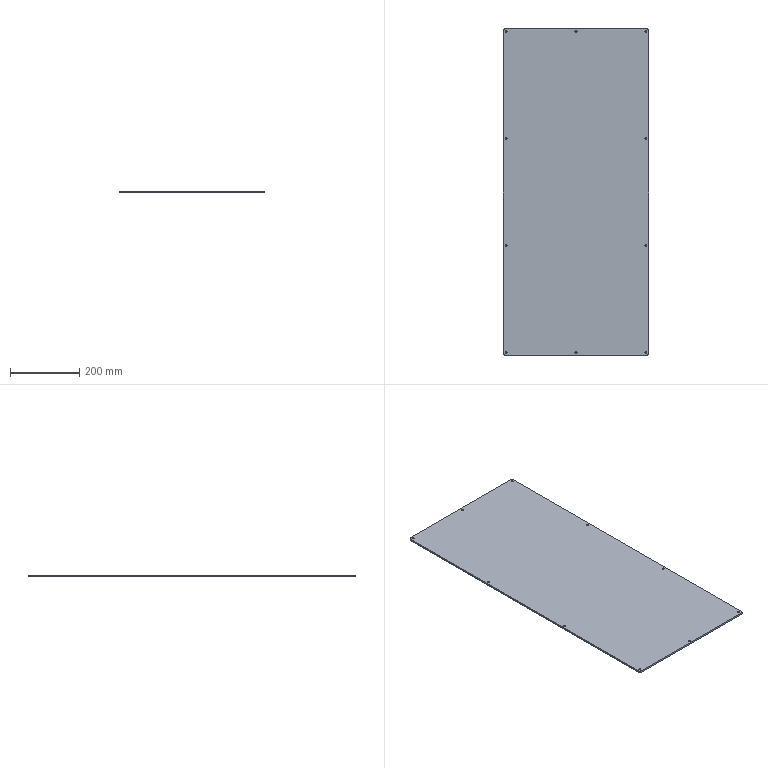Part | NX | features BREP 1 | 1 solid | 30 faces | box 421 x 944 x 5 mm | volume 1985692 mm3 | cylinder 24 | plane 6 | commonest cylinder face diameters 5.8 x20 10 x4
STEP:
#1=CARTESIAN_POINT('',(-205.5,472.,5.));
#2=VERTEX_POINT('',#1);
#3=CARTESIAN_POINT('',(-210.5,467.,5.));
#4=VERTEX_POINT('',#3);
#5=CARTESIAN_POINT('',(-205.5,467.,5.));
#6=DIRECTION('',(0.,0.,1.));
#7=DIRECTION('',(1.,0.,0.));
#8=AXIS2_PLACEMENT_3D('',#5,#6,#7);
#9=CIRCLE('',#8,5.);
#10=EDGE_CURVE('',#2,#4,#9,.T.);
#11=ORIENTED_EDGE('',*,*,#10,.F.);
#12=CARTESIAN_POINT('',(-205.5,472.,0.));
#13=VERTEX_POINT('',#12);
#14=CARTESIAN_POINT('',(-205.5,472.,5.));
#15=DIRECTION('',(0.,0.,1.));
#16=VECTOR('',#15,1000.);
#17=LINE('',#14,#16);
#18=EDGE_CURVE('',#13,#2,#17,.T.);
#19=ORIENTED_EDGE('',*,*,#18,.F.);
#20=CARTESIAN_POINT('',(-210.5,467.,0.));
#21=VERTEX_POINT('',#20);
#22=CARTESIAN_POINT('',(-205.5,467.,0.));
#23=DIRECTION('',(0.,0.,-1.));
#24=DIRECTION('',(1.,0.,0.));
#25=AXIS2_PLACEMENT_3D('',#22,#23,#24);
#26=CIRCLE('',#25,5.);
#27=EDGE_CURVE('',#21,#13,#26,.T.);
#28=ORIENTED_EDGE('',*,*,#27,.F.);
#29=CARTESIAN_POINT('',(-210.5,467.,5.));
#30=DIRECTION('',(0.,0.,-1.));
#31=VECTOR('',#30,1000.);
#32=LINE('',#29,#31);
#33=EDGE_CURVE('',#4,#21,#32,.T.);
#34=ORIENTED_EDGE('',*,*,#33,.F.);
#35=EDGE_LOOP('',(#11,#19,#28,#34));
#36=FACE_BOUND('',#35,.T.);
#37=CARTESIAN_POINT('',(-205.5,467.,5.));
#38=DIRECTION('',(0.,0.,-1.));
#39=DIRECTION('',(-1.,0.,0.));
#40=AXIS2_PLACEMENT_3D('',#37,#38,#39);
#41=CYLINDRICAL_SURFACE('',#40,5.);
#42=ADVANCED_FACE('',(#36),#41,.T.);
#43=CARTESIAN_POINT('',(210.5,467.,5.));
#44=VERTEX_POINT('',#43);
#45=CARTESIAN_POINT('',(205.5,472.,5.));
#46=VERTEX_POINT('',#45);
#47=CARTESIAN_POINT('',(205.5,467.,5.));
#48=DIRECTION('',(0.,0.,1.));
#49=DIRECTION('',(1.,0.,0.));
#50=AXIS2_PLACEMENT_3D('',#47,#48,#49);
#51=CIRCLE('',#50,5.);
#52=EDGE_CURVE('',#44,#46,#51,.T.);
#53=ORIENTED_EDGE('',*,*,#52,.F.);
#54=CARTESIAN_POINT('',(210.5,467.,0.));
#55=VERTEX_POINT('',#54);
#56=CARTESIAN_POINT('',(210.5,467.,5.));
#57=DIRECTION('',(0.,0.,1.));
#58=VECTOR('',#57,1000.);
#59=LINE('',#56,#58);
#60=EDGE_CURVE('',#55,#44,#59,.T.);
#61=ORIENTED_EDGE('',*,*,#60,.F.);
#62=CARTESIAN_POINT('',(205.5,472.,0.));
#63=VERTEX_POINT('',#62);
#64=CARTESIAN_POINT('',(205.5,467.,0.));
#65=DIRECTION('',(0.,0.,-1.));
#66=DIRECTION('',(1.,0.,0.));
#67=AXIS2_PLACEMENT_3D('',#64,#65,#66);
#68=CIRCLE('',#67,5.);
#69=EDGE_CURVE('',#63,#55,#68,.T.);
#70=ORIENTED_EDGE('',*,*,#69,.F.);
#71=CARTESIAN_POINT('',(205.5,472.,5.));
#72=DIRECTION('',(0.,0.,-1.));
#73=VECTOR('',#72,1000.);
#74=LINE('',#71,#73);
#75=EDGE_CURVE('',#46,#63,#74,.T.);
#76=ORIENTED_EDGE('',*,*,#75,.F.);
#77=EDGE_LOOP('',(#53,#61,#70,#76));
#78=FACE_BOUND('',#77,.T.);
#79=CARTESIAN_POINT('',(205.5,467.,5.));
#80=DIRECTION('',(0.,0.,-1.));
#81=DIRECTION('',(-1.,0.,0.));
#82=AXIS2_PLACEMENT_3D('',#79,#80,#81);
#83=CYLINDRICAL_SURFACE('',#82,5.);
#84=ADVANCED_FACE('',(#78),#83,.T.);
#85=CARTESIAN_POINT('',(205.5,-472.,5.));
#86=VERTEX_POINT('',#85);
#87=CARTESIAN_POINT('',(210.5,-467.,5.));
#88=VERTEX_POINT('',#87);
#89=CARTESIAN_POINT('',(205.5,-467.,5.));
#90=DIRECTION('',(0.,0.,1.));
#91=DIRECTION('',(1.,0.,0.));
#92=AXIS2_PLACEMENT_3D('',#89,#90,#91);
#93=CIRCLE('',#92,5.);
#94=EDGE_CURVE('',#86,#88,#93,.T.);
#95=ORIENTED_EDGE('',*,*,#94,.F.);
#96=CARTESIAN_POINT('',(205.5,-472.,0.));
#97=VERTEX_POINT('',#96);
#98=CARTESIAN_POINT('',(205.5,-472.,5.));
#99=DIRECTION('',(0.,0.,1.));
#100=VECTOR('',#99,1000.);
#101=LINE('',#98,#100);
#102=EDGE_CURVE('',#97,#86,#101,.T.);
#103=ORIENTED_EDGE('',*,*,#102,.F.);
#104=CARTESIAN_POINT('',(210.5,-467.,0.));
#105=VERTEX_POINT('',#104);
#106=CARTESIAN_POINT('',(205.5,-467.,0.));
#107=DIRECTION('',(0.,0.,-1.));
#108=DIRECTION('',(1.,0.,0.));
#109=AXIS2_PLACEMENT_3D('',#106,#107,#108);
#110=CIRCLE('',#109,5.);
#111=EDGE_CURVE('',#105,#97,#110,.T.);
#112=ORIENTED_EDGE('',*,*,#111,.F.);
#113=CARTESIAN_POINT('',(210.5,-467.,5.));
#114=DIRECTION('',(0.,0.,-1.));
#115=VECTOR('',#114,1000.);
#116=LINE('',#113,#115);
#117=EDGE_CURVE('',#88,#105,#116,.T.);
#118=ORIENTED_EDGE('',*,*,#117,.F.);
#119=EDGE_LOOP('',(#95,#103,#112,#118));
#120=FACE_BOUND('',#119,.T.);
#121=CARTESIAN_POINT('',(205.5,-467.,5.));
#122=DIRECTION('',(0.,0.,-1.));
#123=DIRECTION('',(-1.,0.,0.));
#124=AXIS2_PLACEMENT_3D('',#121,#122,#123);
#125=CYLINDRICAL_SURFACE('',#124,5.);
#126=ADVANCED_FACE('',(#120),#125,.T.);
#127=CARTESIAN_POINT('',(-210.5,-467.,5.));
#128=VERTEX_POINT('',#127);
#129=CARTESIAN_POINT('',(-205.5,-472.,5.));
#130=VERTEX_POINT('',#129);
#131=CARTESIAN_POINT('',(-205.5,-467.,5.));
#132=DIRECTION('',(0.,0.,1.));
#133=DIRECTION('',(1.,0.,0.));
#134=AXIS2_PLACEMENT_3D('',#131,#132,#133);
#135=CIRCLE('',#134,5.);
#136=EDGE_CURVE('',#128,#130,#135,.T.);
#137=ORIENTED_EDGE('',*,*,#136,.F.);
#138=CARTESIAN_POINT('',(-210.5,-467.,0.));
#139=VERTEX_POINT('',#138);
#140=CARTESIAN_POINT('',(-210.5,-467.,5.));
#141=DIRECTION('',(0.,0.,1.));
#142=VECTOR('',#141,1000.);
#143=LINE('',#140,#142);
#144=EDGE_CURVE('',#139,#128,#143,.T.);
#145=ORIENTED_EDGE('',*,*,#144,.F.);
#146=CARTESIAN_POINT('',(-205.5,-472.,0.));
#147=VERTEX_POINT('',#146);
#148=CARTESIAN_POINT('',(-205.5,-467.,0.));
#149=DIRECTION('',(0.,0.,-1.));
#150=DIRECTION('',(1.,0.,0.));
#151=AXIS2_PLACEMENT_3D('',#148,#149,#150);
#152=CIRCLE('',#151,5.);
#153=EDGE_CURVE('',#147,#139,#152,.T.);
#154=ORIENTED_EDGE('',*,*,#153,.F.);
#155=CARTESIAN_POINT('',(-205.5,-472.,5.));
#156=DIRECTION('',(0.,0.,-1.));
#157=VECTOR('',#156,1000.);
#158=LINE('',#155,#157);
#159=EDGE_CURVE('',#130,#147,#158,.T.);
#160=ORIENTED_EDGE('',*,*,#159,.F.);
#161=EDGE_LOOP('',(#137,#145,#154,#160));
#162=FACE_BOUND('',#161,.T.);
#163=CARTESIAN_POINT('',(-205.5,-467.,5.));
#164=DIRECTION('',(0.,0.,-1.));
#165=DIRECTION('',(-1.,0.,0.));
#166=AXIS2_PLACEMENT_3D('',#163,#164,#165);
#167=CYLINDRICAL_SURFACE('',#166,5.);
#168=ADVANCED_FACE('',(#162),#167,.T.);
#169=CARTESIAN_POINT('',(199.6,-464.,5.));
#170=VERTEX_POINT('',#169);
#171=CARTESIAN_POINT('',(199.6,-464.,0.));
#172=VERTEX_POINT('',#171);
#173=CARTESIAN_POINT('',(199.6,-464.,0.));
#174=DIRECTION('',(0.,0.,1.));
#175=VECTOR('',#174,1000.);
#176=LINE('',#173,#175);
#177=EDGE_CURVE('',#170,#172,#176,.F.);
#178=ORIENTED_EDGE('',*,*,#177,.T.);
#179=CARTESIAN_POINT('',(205.4,-464.,0.));
#180=VERTEX_POINT('',#179);
#181=CARTESIAN_POINT('',(202.5,-464.,0.));
#182=DIRECTION('',(0.,0.,1.));
#183=DIRECTION('',(1.,0.,0.));
#184=AXIS2_PLACEMENT_3D('',#181,#182,#183);
#185=CIRCLE('',#184,2.9);
#186=EDGE_CURVE('',#180,#172,#185,.T.);
#187=ORIENTED_EDGE('',*,*,#186,.F.);
#188=CARTESIAN_POINT('',(205.4,-464.,5.));
#189=VERTEX_POINT('',#188);
#190=CARTESIAN_POINT('',(205.4,-464.,0.));
#191=DIRECTION('',(0.,0.,1.));
#192=VECTOR('',#191,1000.);
#193=LINE('',#190,#192);
#194=EDGE_CURVE('',#189,#180,#193,.F.);
#195=ORIENTED_EDGE('',*,*,#194,.F.);
#196=CARTESIAN_POINT('',(202.5,-464.,5.));
#197=DIRECTION('',(0.,0.,1.));
#198=DIRECTION('',(1.,0.,0.));
#199=AXIS2_PLACEMENT_3D('',#196,#197,#198);
#200=CIRCLE('',#199,2.9);
#201=EDGE_CURVE('',#189,#170,#200,.T.);
#202=ORIENTED_EDGE('',*,*,#201,.T.);
#203=EDGE_LOOP('',(#178,#187,#195,#202));
#204=FACE_BOUND('',#203,.T.);
#205=CARTESIAN_POINT('',(202.5,-464.,0.));
#206=DIRECTION('',(0.,0.,1.));
#207=DIRECTION('',(1.,0.,0.));
#208=AXIS2_PLACEMENT_3D('',#205,#206,#207);
#209=CYLINDRICAL_SURFACE('',#208,2.9);
#210=ADVANCED_FACE('',(#204),#209,.F.);
#211=CARTESIAN_POINT('',(199.6,154.667,5.));
#212=VERTEX_POINT('',#211);
#213=CARTESIAN_POINT('',(199.6,154.667,0.));
#214=VERTEX_POINT('',#213);
#215=CARTESIAN_POINT('',(199.6,154.667,0.));
#216=DIRECTION('',(0.,0.,1.));
#217=VECTOR('',#216,1000.);
#218=LINE('',#215,#217);
#219=EDGE_CURVE('',#212,#214,#218,.F.);
#220=ORIENTED_EDGE('',*,*,#219,.T.);
#221=CARTESIAN_POINT('',(205.4,154.667,0.));
#222=VERTEX_POINT('',#221);
#223=CARTESIAN_POINT('',(202.5,154.667,0.));
#224=DIRECTION('',(0.,0.,1.));
#225=DIRECTION('',(1.,0.,0.));
#226=AXIS2_PLACEMENT_3D('',#223,#224,#225);
#227=CIRCLE('',#226,2.9);
#228=EDGE_CURVE('',#222,#214,#227,.T.);
#229=ORIENTED_EDGE('',*,*,#228,.F.);
#230=CARTESIAN_POINT('',(205.4,154.667,5.));
#231=VERTEX_POINT('',#230);
#232=CARTESIAN_POINT('',(205.4,154.667,0.));
#233=DIRECTION('',(0.,0.,1.));
#234=VECTOR('',#233,1000.);
#235=LINE('',#232,#234);
#236=EDGE_CURVE('',#231,#222,#235,.F.);
#237=ORIENTED_EDGE('',*,*,#236,.F.);
#238=CARTESIAN_POINT('',(202.5,154.667,5.));
#239=DIRECTION('',(0.,0.,1.));
#240=DIRECTION('',(1.,0.,0.));
#241=AXIS2_PLACEMENT_3D('',#238,#239,#240);
#242=CIRCLE('',#241,2.9);
#243=EDGE_CURVE('',#231,#212,#242,.T.);
#244=ORIENTED_EDGE('',*,*,#243,.T.);
#245=EDGE_LOOP('',(#220,#229,#237,#244));
#246=FACE_BOUND('',#245,.T.);
#247=CARTESIAN_POINT('',(202.5,154.667,0.));
#248=DIRECTION('',(0.,0.,1.));
#249=DIRECTION('',(1.,0.,0.));
#250=AXIS2_PLACEMENT_3D('',#247,#248,#249);
#251=CYLINDRICAL_SURFACE('',#250,2.9);
#252=ADVANCED_FACE('',(#246),#251,.F.);
#253=CARTESIAN_POINT('',(199.6,-154.667,5.));
#254=VERTEX_POINT('',#253);
#255=CARTESIAN_POINT('',(199.6,-154.667,0.));
#256=VERTEX_POINT('',#255);
#257=CARTESIAN_POINT('',(199.6,-154.667,0.));
#258=DIRECTION('',(0.,0.,1.));
#259=VECTOR('',#258,1000.);
#260=LINE('',#257,#259);
#261=EDGE_CURVE('',#254,#256,#260,.F.);
#262=ORIENTED_EDGE('',*,*,#261,.T.);
#263=CARTESIAN_POINT('',(205.4,-154.667,0.));
#264=VERTEX_POINT('',#263);
#265=CARTESIAN_POINT('',(202.5,-154.667,0.));
#266=DIRECTION('',(0.,0.,1.));
#267=DIRECTION('',(1.,0.,0.));
#268=AXIS2_PLACEMENT_3D('',#265,#266,#267);
#269=CIRCLE('',#268,2.9);
#270=EDGE_CURVE('',#264,#256,#269,.T.);
#271=ORIENTED_EDGE('',*,*,#270,.F.);
#272=CARTESIAN_POINT('',(205.4,-154.667,5.));
#273=VERTEX_POINT('',#272);
#274=CARTESIAN_POINT('',(205.4,-154.667,0.));
#275=DIRECTION('',(0.,0.,1.));
#276=VECTOR('',#275,1000.);
#277=LINE('',#274,#276);
#278=EDGE_CURVE('',#273,#264,#277,.F.);
#279=ORIENTED_EDGE('',*,*,#278,.F.);
#280=CARTESIAN_POINT('',(202.5,-154.667,5.));
#281=DIRECTION('',(0.,0.,1.));
#282=DIRECTION('',(1.,0.,0.));
#283=AXIS2_PLACEMENT_3D('',#280,#281,#282);
#284=CIRCLE('',#283,2.9);
#285=EDGE_CURVE('',#273,#254,#284,.T.);
#286=ORIENTED_EDGE('',*,*,#285,.T.);
#287=EDGE_LOOP('',(#262,#271,#279,#286));
#288=FACE_BOUND('',#287,.T.);
#289=CARTESIAN_POINT('',(202.5,-154.667,0.));
#290=DIRECTION('',(0.,0.,1.));
#291=DIRECTION('',(1.,0.,0.));
#292=AXIS2_PLACEMENT_3D('',#289,#290,#291);
#293=CYLINDRICAL_SURFACE('',#292,2.9);
#294=ADVANCED_FACE('',(#288),#293,.F.);
#295=CARTESIAN_POINT('',(-205.4,154.667,5.));
#296=VERTEX_POINT('',#295);
#297=CARTESIAN_POINT('',(-205.4,154.667,0.));
#298=VERTEX_POINT('',#297);
#299=CARTESIAN_POINT('',(-205.4,154.667,0.));
#300=DIRECTION('',(0.,0.,1.));
#301=VECTOR('',#300,1000.);
#302=LINE('',#299,#301);
#303=EDGE_CURVE('',#296,#298,#302,.F.);
#304=ORIENTED_EDGE('',*,*,#303,.T.);
#305=CARTESIAN_POINT('',(-199.6,154.667,0.));
#306=VERTEX_POINT('',#305);
#307=CARTESIAN_POINT('',(-202.5,154.667,0.));
#308=DIRECTION('',(0.,0.,1.));
#309=DIRECTION('',(1.,0.,0.));
#310=AXIS2_PLACEMENT_3D('',#307,#308,#309);
#311=CIRCLE('',#310,2.9);
#312=EDGE_CURVE('',#306,#298,#311,.T.);
#313=ORIENTED_EDGE('',*,*,#312,.F.);
#314=CARTESIAN_POINT('',(-199.6,154.667,5.));
#315=VERTEX_POINT('',#314);
#316=CARTESIAN_POINT('',(-199.6,154.667,0.));
#317=DIRECTION('',(0.,0.,1.));
#318=VECTOR('',#317,1000.);
#319=LINE('',#316,#318);
#320=EDGE_CURVE('',#315,#306,#319,.F.);
#321=ORIENTED_EDGE('',*,*,#320,.F.);
#322=CARTESIAN_POINT('',(-202.5,154.667,5.));
#323=DIRECTION('',(0.,0.,1.));
#324=DIRECTION('',(1.,0.,0.));
#325=AXIS2_PLACEMENT_3D('',#322,#323,#324);
#326=CIRCLE('',#325,2.9);
#327=EDGE_CURVE('',#315,#296,#326,.T.);
#328=ORIENTED_EDGE('',*,*,#327,.T.);
#329=EDGE_LOOP('',(#304,#313,#321,#328));
#330=FACE_BOUND('',#329,.T.);
#331=CARTESIAN_POINT('',(-202.5,154.667,0.));
#332=DIRECTION('',(0.,0.,1.));
#333=DIRECTION('',(1.,0.,0.));
#334=AXIS2_PLACEMENT_3D('',#331,#332,#333);
#335=CYLINDRICAL_SURFACE('',#334,2.9);
#336=ADVANCED_FACE('',(#330),#335,.F.);
#337=CARTESIAN_POINT('',(-2.9,-464.,5.));
#338=VERTEX_POINT('',#337);
#339=CARTESIAN_POINT('',(-2.9,-464.,0.));
#340=VERTEX_POINT('',#339);
#341=CARTESIAN_POINT('',(-2.9,-464.,0.));
#342=DIRECTION('',(0.,0.,1.));
#343=VECTOR('',#342,1000.);
#344=LINE('',#341,#343);
#345=EDGE_CURVE('',#338,#340,#344,.F.);
#346=ORIENTED_EDGE('',*,*,#345,.T.);
#347=CARTESIAN_POINT('',(2.9,-464.,0.));
#348=VERTEX_POINT('',#347);
#349=CARTESIAN_POINT('',(0.,-464.,0.));
#350=DIRECTION('',(0.,0.,1.));
#351=DIRECTION('',(1.,0.,0.));
#352=AXIS2_PLACEMENT_3D('',#349,#350,#351);
#353=CIRCLE('',#352,2.9);
#354=EDGE_CURVE('',#348,#340,#353,.T.);
#355=ORIENTED_EDGE('',*,*,#354,.F.);
#356=CARTESIAN_POINT('',(2.9,-464.,5.));
#357=VERTEX_POINT('',#356);
#358=CARTESIAN_POINT('',(2.9,-464.,0.));
#359=DIRECTION('',(0.,0.,1.));
#360=VECTOR('',#359,1000.);
#361=LINE('',#358,#360);
#362=EDGE_CURVE('',#357,#348,#361,.F.);
#363=ORIENTED_EDGE('',*,*,#362,.F.);
#364=CARTESIAN_POINT('',(0.,-464.,5.));
#365=DIRECTION('',(0.,0.,1.));
#366=DIRECTION('',(1.,0.,0.));
#367=AXIS2_PLACEMENT_3D('',#364,#365,#366);
#368=CIRCLE('',#367,2.9);
#369=EDGE_CURVE('',#357,#338,#368,.T.);
#370=ORIENTED_EDGE('',*,*,#369,.T.);
#371=EDGE_LOOP('',(#346,#355,#363,#370));
#372=FACE_BOUND('',#371,.T.);
#373=CARTESIAN_POINT('',(0.,-464.,0.));
#374=DIRECTION('',(0.,0.,1.));
#375=DIRECTION('',(1.,0.,0.));
#376=AXIS2_PLACEMENT_3D('',#373,#374,#375);
#377=CYLINDRICAL_SURFACE('',#376,2.9);
#378=ADVANCED_FACE('',(#372),#377,.F.);
#379=CARTESIAN_POINT('',(-205.4,-464.,5.));
#380=VERTEX_POINT('',#379);
#381=CARTESIAN_POINT('',(-205.4,-464.,0.));
#382=VERTEX_POINT('',#381);
#383=CARTESIAN_POINT('',(-205.4,-464.,0.));
#384=DIRECTION('',(0.,0.,1.));
#385=VECTOR('',#384,1000.);
#386=LINE('',#383,#385);
#387=EDGE_CURVE('',#380,#382,#386,.F.);
#388=ORIENTED_EDGE('',*,*,#387,.T.);
#389=CARTESIAN_POINT('',(-199.6,-464.,0.));
#390=VERTEX_POINT('',#389);
#391=CARTESIAN_POINT('',(-202.5,-464.,0.));
#392=DIRECTION('',(0.,0.,1.));
#393=DIRECTION('',(1.,0.,0.));
#394=AXIS2_PLACEMENT_3D('',#391,#392,#393);
#395=CIRCLE('',#394,2.9);
#396=EDGE_CURVE('',#390,#382,#395,.T.);
#397=ORIENTED_EDGE('',*,*,#396,.F.);
#398=CARTESIAN_POINT('',(-199.6,-464.,5.));
#399=VERTEX_POINT('',#398);
#400=CARTESIAN_POINT('',(-199.6,-464.,0.));
#401=DIRECTION('',(0.,0.,1.));
#402=VECTOR('',#401,1000.);
#403=LINE('',#400,#402);
#404=EDGE_CURVE('',#399,#390,#403,.F.);
#405=ORIENTED_EDGE('',*,*,#404,.F.);
#406=CARTESIAN_POINT('',(-202.5,-464.,5.));
#407=DIRECTION('',(0.,0.,1.));
#408=DIRECTION('',(1.,0.,0.));
#409=AXIS2_PLACEMENT_3D('',#406,#407,#408);
#410=CIRCLE('',#409,2.9);
#411=EDGE_CURVE('',#399,#380,#410,.T.);
#412=ORIENTED_EDGE('',*,*,#411,.T.);
#413=EDGE_LOOP('',(#388,#397,#405,#412));
#414=FACE_BOUND('',#413,.T.);
#415=CARTESIAN_POINT('',(-202.5,-464.,0.));
#416=DIRECTION('',(0.,0.,1.));
#417=DIRECTION('',(1.,0.,0.));
#418=AXIS2_PLACEMENT_3D('',#415,#416,#417);
#419=CYLINDRICAL_SURFACE('',#418,2.9);
#420=ADVANCED_FACE('',(#414),#419,.F.);
#421=CARTESIAN_POINT('',(199.6,464.,5.));
#422=VERTEX_POINT('',#421);
#423=CARTESIAN_POINT('',(199.6,464.,0.));
#424=VERTEX_POINT('',#423);
#425=CARTESIAN_POINT('',(199.6,464.,0.));
#426=DIRECTION('',(0.,0.,1.));
#427=VECTOR('',#426,1000.);
#428=LINE('',#425,#427);
#429=EDGE_CURVE('',#422,#424,#428,.F.);
#430=ORIENTED_EDGE('',*,*,#429,.T.);
#431=CARTESIAN_POINT('',(205.4,464.,0.));
#432=VERTEX_POINT('',#431);
#433=CARTESIAN_POINT('',(202.5,464.,0.));
#434=DIRECTION('',(0.,0.,1.));
#435=DIRECTION('',(1.,0.,0.));
#436=AXIS2_PLACEMENT_3D('',#433,#434,#435);
#437=CIRCLE('',#436,2.9);
#438=EDGE_CURVE('',#432,#424,#437,.T.);
#439=ORIENTED_EDGE('',*,*,#438,.F.);
#440=CARTESIAN_POINT('',(205.4,464.,5.));
#441=VERTEX_POINT('',#440);
#442=CARTESIAN_POINT('',(205.4,464.,0.));
#443=DIRECTION('',(0.,0.,1.));
#444=VECTOR('',#443,1000.);
#445=LINE('',#442,#444);
#446=EDGE_CURVE('',#441,#432,#445,.F.);
#447=ORIENTED_EDGE('',*,*,#446,.F.);
#448=CARTESIAN_POINT('',(202.5,464.,5.));
#449=DIRECTION('',(0.,0.,1.));
#450=DIRECTION('',(1.,0.,0.));
#451=AXIS2_PLACEMENT_3D('',#448,#449,#450);
#452=CIRCLE('',#451,2.9);
#453=EDGE_CURVE('',#441,#422,#452,.T.);
#454=ORIENTED_EDGE('',*,*,#453,.T.);
#455=EDGE_LOOP('',(#430,#439,#447,#454));
#456=FACE_BOUND('',#455,.T.);
#457=CARTESIAN_POINT('',(202.5,464.,0.));
#458=DIRECTION('',(0.,0.,1.));
#459=DIRECTION('',(1.,0.,0.));
#460=AXIS2_PLACEMENT_3D('',#457,#458,#459);
#461=CYLINDRICAL_SURFACE('',#460,2.9);
#462=ADVANCED_FACE('',(#456),#461,.F.);
#463=CARTESIAN_POINT('',(-2.9,464.,5.));
#464=VERTEX_POINT('',#463);
#465=CARTESIAN_POINT('',(-2.9,464.,0.));
#466=VERTEX_POINT('',#465);
#467=CARTESIAN_POINT('',(-2.9,464.,0.));
#468=DIRECTION('',(0.,0.,1.));
#469=VECTOR('',#468,1000.);
#470=LINE('',#467,#469);
#471=EDGE_CURVE('',#464,#466,#470,.F.);
#472=ORIENTED_EDGE('',*,*,#471,.T.);
#473=CARTESIAN_POINT('',(2.9,464.,0.));
#474=VERTEX_POINT('',#473);
#475=CARTESIAN_POINT('',(0.,464.,0.));
#476=DIRECTION('',(0.,0.,1.));
#477=DIRECTION('',(1.,0.,0.));
#478=AXIS2_PLACEMENT_3D('',#475,#476,#477);
#479=CIRCLE('',#478,2.9);
#480=EDGE_CURVE('',#474,#466,#479,.T.);
#481=ORIENTED_EDGE('',*,*,#480,.F.);
#482=CARTESIAN_POINT('',(2.9,464.,5.));
#483=VERTEX_POINT('',#482);
#484=CARTESIAN_POINT('',(2.9,464.,0.));
#485=DIRECTION('',(0.,0.,1.));
#486=VECTOR('',#485,1000.);
#487=LINE('',#484,#486);
#488=EDGE_CURVE('',#483,#474,#487,.F.);
#489=ORIENTED_EDGE('',*,*,#488,.F.);
#490=CARTESIAN_POINT('',(0.,464.,5.));
#491=DIRECTION('',(0.,0.,1.));
#492=DIRECTION('',(1.,0.,0.));
#493=AXIS2_PLACEMENT_3D('',#490,#491,#492);
#494=CIRCLE('',#493,2.9);
#495=EDGE_CURVE('',#483,#464,#494,.T.);
#496=ORIENTED_EDGE('',*,*,#495,.T.);
#497=EDGE_LOOP('',(#472,#481,#489,#496));
#498=FACE_BOUND('',#497,.T.);
#499=CARTESIAN_POINT('',(0.,464.,0.));
#500=DIRECTION('',(0.,0.,1.));
#501=DIRECTION('',(1.,0.,0.));
#502=AXIS2_PLACEMENT_3D('',#499,#500,#501);
#503=CYLINDRICAL_SURFACE('',#502,2.9);
#504=ADVANCED_FACE('',(#498),#503,.F.);
#505=CARTESIAN_POINT('',(-205.4,-154.667,5.));
#506=VERTEX_POINT('',#505);
#507=CARTESIAN_POINT('',(-205.4,-154.667,0.));
#508=VERTEX_POINT('',#507);
#509=CARTESIAN_POINT('',(-205.4,-154.667,0.));
#510=DIRECTION('',(0.,0.,1.));
#511=VECTOR('',#510,1000.);
#512=LINE('',#509,#511);
#513=EDGE_CURVE('',#506,#508,#512,.F.);
#514=ORIENTED_EDGE('',*,*,#513,.T.);
#515=CARTESIAN_POINT('',(-199.6,-154.667,0.));
#516=VERTEX_POINT('',#515);
#517=CARTESIAN_POINT('',(-202.5,-154.667,0.));
#518=DIRECTION('',(0.,0.,1.));
#519=DIRECTION('',(1.,0.,0.));
#520=AXIS2_PLACEMENT_3D('',#517,#518,#519);
#521=CIRCLE('',#520,2.9);
#522=EDGE_CURVE('',#516,#508,#521,.T.);
#523=ORIENTED_EDGE('',*,*,#522,.F.);
#524=CARTESIAN_POINT('',(-199.6,-154.667,5.));
#525=VERTEX_POINT('',#524);
#526=CARTESIAN_POINT('',(-199.6,-154.667,0.));
#527=DIRECTION('',(0.,0.,1.));
#528=VECTOR('',#527,1000.);
#529=LINE('',#526,#528);
#530=EDGE_CURVE('',#525,#516,#529,.F.);
#531=ORIENTED_EDGE('',*,*,#530,.F.);
#532=CARTESIAN_POINT('',(-202.5,-154.667,5.));
#533=DIRECTION('',(0.,0.,1.));
#534=DIRECTION('',(1.,0.,0.));
#535=AXIS2_PLACEMENT_3D('',#532,#533,#534);
#536=CIRCLE('',#535,2.9);
#537=EDGE_CURVE('',#525,#506,#536,.T.);
#538=ORIENTED_EDGE('',*,*,#537,.T.);
#539=EDGE_LOOP('',(#514,#523,#531,#538));
#540=FACE_BOUND('',#539,.T.);
#541=CARTESIAN_POINT('',(-202.5,-154.667,0.));
#542=DIRECTION('',(0.,0.,1.));
#543=DIRECTION('',(1.,0.,0.));
#544=AXIS2_PLACEMENT_3D('',#541,#542,#543);
#545=CYLINDRICAL_SURFACE('',#544,2.9);
#546=ADVANCED_FACE('',(#540),#545,.F.);
#547=CARTESIAN_POINT('',(-205.4,464.,5.));
#548=VERTEX_POINT('',#547);
#549=CARTESIAN_POINT('',(-205.4,464.,0.));
#550=VERTEX_POINT('',#549);
#551=CARTESIAN_POINT('',(-205.4,464.,0.));
#552=DIRECTION('',(0.,0.,1.));
#553=VECTOR('',#552,1000.);
#554=LINE('',#551,#553);
#555=EDGE_CURVE('',#548,#550,#554,.F.);
#556=ORIENTED_EDGE('',*,*,#555,.T.);
#557=CARTESIAN_POINT('',(-199.6,464.,0.));
#558=VERTEX_POINT('',#557);
#559=CARTESIAN_POINT('',(-202.5,464.,0.));
#560=DIRECTION('',(0.,0.,1.));
#561=DIRECTION('',(1.,0.,0.));
#562=AXIS2_PLACEMENT_3D('',#559,#560,#561);
#563=CIRCLE('',#562,2.9);
#564=EDGE_CURVE('',#558,#550,#563,.T.);
#565=ORIENTED_EDGE('',*,*,#564,.F.);
#566=CARTESIAN_POINT('',(-199.6,464.,5.));
#567=VERTEX_POINT('',#566);
#568=CARTESIAN_POINT('',(-199.6,464.,0.));
#569=DIRECTION('',(0.,0.,1.));
#570=VECTOR('',#569,1000.);
#571=LINE('',#568,#570);
#572=EDGE_CURVE('',#567,#558,#571,.F.);
#573=ORIENTED_EDGE('',*,*,#572,.F.);
#574=CARTESIAN_POINT('',(-202.5,464.,5.));
#575=DIRECTION('',(0.,0.,1.));
#576=DIRECTION('',(1.,0.,0.));
#577=AXIS2_PLACEMENT_3D('',#574,#575,#576);
#578=CIRCLE('',#577,2.9);
#579=EDGE_CURVE('',#567,#548,#578,.T.);
#580=ORIENTED_EDGE('',*,*,#579,.T.);
#581=EDGE_LOOP('',(#556,#565,#573,#580));
#582=FACE_BOUND('',#581,.T.);
#583=CARTESIAN_POINT('',(-202.5,464.,0.));
#584=DIRECTION('',(0.,0.,1.));
#585=DIRECTION('',(1.,0.,0.));
#586=AXIS2_PLACEMENT_3D('',#583,#584,#585);
#587=CYLINDRICAL_SURFACE('',#586,2.9);
#588=ADVANCED_FACE('',(#582),#587,.F.);
#589=CARTESIAN_POINT('',(210.5,-472.,0.));
#590=DIRECTION('',(1.,0.,0.));
#591=VECTOR('',#590,1000.);
#592=LINE('',#589,#591);
#593=EDGE_CURVE('',#147,#97,#592,.T.);
#594=ORIENTED_EDGE('',*,*,#593,.F.);
#595=ORIENTED_EDGE('',*,*,#153,.T.);
#596=CARTESIAN_POINT('',(-210.5,-472.,0.));
#597=DIRECTION('',(0.,-1.,0.));
#598=VECTOR('',#597,1000.);
#599=LINE('',#596,#598);
#600=EDGE_CURVE('',#21,#139,#599,.T.);
#601=ORIENTED_EDGE('',*,*,#600,.F.);
#602=ORIENTED_EDGE('',*,*,#27,.T.);
#603=CARTESIAN_POINT('',(210.5,472.,0.));
#604=DIRECTION('',(-1.,0.,0.));
#605=VECTOR('',#604,1000.);
#606=LINE('',#603,#605);
#607=EDGE_CURVE('',#63,#13,#606,.T.);
#608=ORIENTED_EDGE('',*,*,#607,.F.);
#609=ORIENTED_EDGE('',*,*,#69,.T.);
#610=CARTESIAN_POINT('',(210.5,-472.,0.));
#611=DIRECTION('',(0.,1.,0.));
#612=VECTOR('',#611,1000.);
#613=LINE('',#610,#612);
#614=EDGE_CURVE('',#105,#55,#613,.T.);
#615=ORIENTED_EDGE('',*,*,#614,.F.);
#616=ORIENTED_EDGE('',*,*,#111,.T.);
#617=EDGE_LOOP('',(#594,#595,#601,#602,#608,#609,#615,#616));
#618=FACE_BOUND('',#617,.T.);
#619=ORIENTED_EDGE('',*,*,#564,.T.);
#620=CARTESIAN_POINT('',(-202.5,464.,0.));
#621=DIRECTION('',(0.,0.,1.));
#622=DIRECTION('',(1.,0.,0.));
#623=AXIS2_PLACEMENT_3D('',#620,#621,#622);
#624=CIRCLE('',#623,2.9);
#625=EDGE_CURVE('',#550,#558,#624,.T.);
#626=ORIENTED_EDGE('',*,*,#625,.T.);
#627=EDGE_LOOP('',(#619,#626));
#628=FACE_BOUND('',#627,.T.);
#629=ORIENTED_EDGE('',*,*,#522,.T.);
#630=CARTESIAN_POINT('',(-202.5,-154.667,0.));
#631=DIRECTION('',(0.,0.,1.));
#632=DIRECTION('',(1.,0.,0.));
#633=AXIS2_PLACEMENT_3D('',#630,#631,#632);
#634=CIRCLE('',#633,2.9);
#635=EDGE_CURVE('',#508,#516,#634,.T.);
#636=ORIENTED_EDGE('',*,*,#635,.T.);
#637=EDGE_LOOP('',(#629,#636));
#638=FACE_BOUND('',#637,.T.);
#639=ORIENTED_EDGE('',*,*,#480,.T.);
#640=CARTESIAN_POINT('',(0.,464.,0.));
#641=DIRECTION('',(0.,0.,1.));
#642=DIRECTION('',(1.,0.,0.));
#643=AXIS2_PLACEMENT_3D('',#640,#641,#642);
#644=CIRCLE('',#643,2.9);
#645=EDGE_CURVE('',#466,#474,#644,.T.);
#646=ORIENTED_EDGE('',*,*,#645,.T.);
#647=EDGE_LOOP('',(#639,#646));
#648=FACE_BOUND('',#647,.T.);
#649=ORIENTED_EDGE('',*,*,#438,.T.);
#650=CARTESIAN_POINT('',(202.5,464.,0.));
#651=DIRECTION('',(0.,0.,1.));
#652=DIRECTION('',(1.,0.,0.));
#653=AXIS2_PLACEMENT_3D('',#650,#651,#652);
#654=CIRCLE('',#653,2.9);
#655=EDGE_CURVE('',#424,#432,#654,.T.);
#656=ORIENTED_EDGE('',*,*,#655,.T.);
#657=EDGE_LOOP('',(#649,#656));
#658=FACE_BOUND('',#657,.T.);
#659=ORIENTED_EDGE('',*,*,#396,.T.);
#660=CARTESIAN_POINT('',(-202.5,-464.,0.));
#661=DIRECTION('',(0.,0.,1.));
#662=DIRECTION('',(1.,0.,0.));
#663=AXIS2_PLACEMENT_3D('',#660,#661,#662);
#664=CIRCLE('',#663,2.9);
#665=EDGE_CURVE('',#382,#390,#664,.T.);
#666=ORIENTED_EDGE('',*,*,#665,.T.);
#667=EDGE_LOOP('',(#659,#666));
#668=FACE_BOUND('',#667,.T.);
#669=ORIENTED_EDGE('',*,*,#354,.T.);
#670=CARTESIAN_POINT('',(0.,-464.,0.));
#671=DIRECTION('',(0.,0.,1.));
#672=DIRECTION('',(1.,0.,0.));
#673=AXIS2_PLACEMENT_3D('',#670,#671,#672);
#674=CIRCLE('',#673,2.9);
#675=EDGE_CURVE('',#340,#348,#674,.T.);
#676=ORIENTED_EDGE('',*,*,#675,.T.);
#677=EDGE_LOOP('',(#669,#676));
#678=FACE_BOUND('',#677,.T.);
#679=ORIENTED_EDGE('',*,*,#312,.T.);
#680=CARTESIAN_POINT('',(-202.5,154.667,0.));
#681=DIRECTION('',(0.,0.,1.));
#682=DIRECTION('',(1.,0.,0.));
#683=AXIS2_PLACEMENT_3D('',#680,#681,#682);
#684=CIRCLE('',#683,2.9);
#685=EDGE_CURVE('',#298,#306,#684,.T.);
#686=ORIENTED_EDGE('',*,*,#685,.T.);
#687=EDGE_LOOP('',(#679,#686));
#688=FACE_BOUND('',#687,.T.);
#689=ORIENTED_EDGE('',*,*,#270,.T.);
#690=CARTESIAN_POINT('',(202.5,-154.667,0.));
#691=DIRECTION('',(0.,0.,1.));
#692=DIRECTION('',(1.,0.,0.));
#693=AXIS2_PLACEMENT_3D('',#690,#691,#692);
#694=CIRCLE('',#693,2.9);
#695=EDGE_CURVE('',#256,#264,#694,.T.);
#696=ORIENTED_EDGE('',*,*,#695,.T.);
#697=EDGE_LOOP('',(#689,#696));
#698=FACE_BOUND('',#697,.T.);
#699=ORIENTED_EDGE('',*,*,#228,.T.);
#700=CARTESIAN_POINT('',(202.5,154.667,0.));
#701=DIRECTION('',(0.,0.,1.));
#702=DIRECTION('',(1.,0.,0.));
#703=AXIS2_PLACEMENT_3D('',#700,#701,#702);
#704=CIRCLE('',#703,2.9);
#705=EDGE_CURVE('',#214,#222,#704,.T.);
#706=ORIENTED_EDGE('',*,*,#705,.T.);
#707=EDGE_LOOP('',(#699,#706));
#708=FACE_BOUND('',#707,.T.);
#709=ORIENTED_EDGE('',*,*,#186,.T.);
#710=CARTESIAN_POINT('',(202.5,-464.,0.));
#711=DIRECTION('',(0.,0.,1.));
#712=DIRECTION('',(1.,0.,0.));
#713=AXIS2_PLACEMENT_3D('',#710,#711,#712);
#714=CIRCLE('',#713,2.9);
#715=EDGE_CURVE('',#172,#180,#714,.T.);
#716=ORIENTED_EDGE('',*,*,#715,.T.);
#717=EDGE_LOOP('',(#709,#716));
#718=FACE_BOUND('',#717,.T.);
#719=CARTESIAN_POINT('',(0.,0.,0.));
#720=DIRECTION('',(0.,0.,1.));
#721=DIRECTION('',(1.,0.,0.));
#722=AXIS2_PLACEMENT_3D('',#719,#720,#721);
#723=PLANE('',#722);
#724=ADVANCED_FACE('',(#618,#628,#638,#648,#658,#668,#678,#688,#698,#708,#718),#723,.F.);
#725=CARTESIAN_POINT('',(-210.5,-472.,5.));
#726=DIRECTION('',(0.,-1.,0.));
#727=VECTOR('',#726,1000.);
#728=LINE('',#725,#727);
#729=EDGE_CURVE('',#4,#128,#728,.T.);
#730=ORIENTED_EDGE('',*,*,#729,.T.);
#731=ORIENTED_EDGE('',*,*,#136,.T.);
#732=CARTESIAN_POINT('',(210.5,-472.,5.));
#733=DIRECTION('',(1.,0.,0.));
#734=VECTOR('',#733,1000.);
#735=LINE('',#732,#734);
#736=EDGE_CURVE('',#130,#86,#735,.T.);
#737=ORIENTED_EDGE('',*,*,#736,.T.);
#738=ORIENTED_EDGE('',*,*,#94,.T.);
#739=CARTESIAN_POINT('',(210.5,-472.,5.));
#740=DIRECTION('',(0.,1.,0.));
#741=VECTOR('',#740,1000.);
#742=LINE('',#739,#741);
#743=EDGE_CURVE('',#88,#44,#742,.T.);
#744=ORIENTED_EDGE('',*,*,#743,.T.);
#745=ORIENTED_EDGE('',*,*,#52,.T.);
#746=CARTESIAN_POINT('',(210.5,472.,5.));
#747=DIRECTION('',(-1.,0.,0.));
#748=VECTOR('',#747,1000.);
#749=LINE('',#746,#748);
#750=EDGE_CURVE('',#46,#2,#749,.T.);
#751=ORIENTED_EDGE('',*,*,#750,.T.);
#752=ORIENTED_EDGE('',*,*,#10,.T.);
#753=EDGE_LOOP('',(#730,#731,#737,#738,#744,#745,#751,#752));
#754=FACE_BOUND('',#753,.T.);
#755=ORIENTED_EDGE('',*,*,#579,.F.);
#756=CARTESIAN_POINT('',(-202.5,464.,5.));
#757=DIRECTION('',(0.,0.,1.));
#758=DIRECTION('',(1.,0.,0.));
#759=AXIS2_PLACEMENT_3D('',#756,#757,#758);
#760=CIRCLE('',#759,2.9);
#761=EDGE_CURVE('',#548,#567,#760,.T.);
#762=ORIENTED_EDGE('',*,*,#761,.F.);
#763=EDGE_LOOP('',(#755,#762));
#764=FACE_BOUND('',#763,.T.);
#765=ORIENTED_EDGE('',*,*,#537,.F.);
#766=CARTESIAN_POINT('',(-202.5,-154.667,5.));
#767=DIRECTION('',(0.,0.,1.));
#768=DIRECTION('',(1.,0.,0.));
#769=AXIS2_PLACEMENT_3D('',#766,#767,#768);
#770=CIRCLE('',#769,2.9);
#771=EDGE_CURVE('',#506,#525,#770,.T.);
#772=ORIENTED_EDGE('',*,*,#771,.F.);
#773=EDGE_LOOP('',(#765,#772));
#774=FACE_BOUND('',#773,.T.);
#775=ORIENTED_EDGE('',*,*,#495,.F.);
#776=CARTESIAN_POINT('',(0.,464.,5.));
#777=DIRECTION('',(0.,0.,1.));
#778=DIRECTION('',(1.,0.,0.));
#779=AXIS2_PLACEMENT_3D('',#776,#777,#778);
#780=CIRCLE('',#779,2.9);
#781=EDGE_CURVE('',#464,#483,#780,.T.);
#782=ORIENTED_EDGE('',*,*,#781,.F.);
#783=EDGE_LOOP('',(#775,#782));
#784=FACE_BOUND('',#783,.T.);
#785=ORIENTED_EDGE('',*,*,#453,.F.);
#786=CARTESIAN_POINT('',(202.5,464.,5.));
#787=DIRECTION('',(0.,0.,1.));
#788=DIRECTION('',(1.,0.,0.));
#789=AXIS2_PLACEMENT_3D('',#786,#787,#788);
#790=CIRCLE('',#789,2.9);
#791=EDGE_CURVE('',#422,#441,#790,.T.);
#792=ORIENTED_EDGE('',*,*,#791,.F.);
#793=EDGE_LOOP('',(#785,#792));
#794=FACE_BOUND('',#793,.T.);
#795=ORIENTED_EDGE('',*,*,#411,.F.);
#796=CARTESIAN_POINT('',(-202.5,-464.,5.));
#797=DIRECTION('',(0.,0.,1.));
#798=DIRECTION('',(1.,0.,0.));
#799=AXIS2_PLACEMENT_3D('',#796,#797,#798);
#800=CIRCLE('',#799,2.9);
#801=EDGE_CURVE('',#380,#399,#800,.T.);
#802=ORIENTED_EDGE('',*,*,#801,.F.);
#803=EDGE_LOOP('',(#795,#802));
#804=FACE_BOUND('',#803,.T.);
#805=ORIENTED_EDGE('',*,*,#369,.F.);
#806=CARTESIAN_POINT('',(0.,-464.,5.));
#807=DIRECTION('',(0.,0.,1.));
#808=DIRECTION('',(1.,0.,0.));
#809=AXIS2_PLACEMENT_3D('',#806,#807,#808);
#810=CIRCLE('',#809,2.9);
#811=EDGE_CURVE('',#338,#357,#810,.T.);
#812=ORIENTED_EDGE('',*,*,#811,.F.);
#813=EDGE_LOOP('',(#805,#812));
#814=FACE_BOUND('',#813,.T.);
#815=ORIENTED_EDGE('',*,*,#327,.F.);
#816=CARTESIAN_POINT('',(-202.5,154.667,5.));
#817=DIRECTION('',(0.,0.,1.));
#818=DIRECTION('',(1.,0.,0.));
#819=AXIS2_PLACEMENT_3D('',#816,#817,#818);
#820=CIRCLE('',#819,2.9);
#821=EDGE_CURVE('',#296,#315,#820,.T.);
#822=ORIENTED_EDGE('',*,*,#821,.F.);
#823=EDGE_LOOP('',(#815,#822));
#824=FACE_BOUND('',#823,.T.);
#825=ORIENTED_EDGE('',*,*,#285,.F.);
#826=CARTESIAN_POINT('',(202.5,-154.667,5.));
#827=DIRECTION('',(0.,0.,1.));
#828=DIRECTION('',(1.,0.,0.));
#829=AXIS2_PLACEMENT_3D('',#826,#827,#828);
#830=CIRCLE('',#829,2.9);
#831=EDGE_CURVE('',#254,#273,#830,.T.);
#832=ORIENTED_EDGE('',*,*,#831,.F.);
#833=EDGE_LOOP('',(#825,#832));
#834=FACE_BOUND('',#833,.T.);
#835=ORIENTED_EDGE('',*,*,#243,.F.);
#836=CARTESIAN_POINT('',(202.5,154.667,5.));
#837=DIRECTION('',(0.,0.,1.));
#838=DIRECTION('',(1.,0.,0.));
#839=AXIS2_PLACEMENT_3D('',#836,#837,#838);
#840=CIRCLE('',#839,2.9);
#841=EDGE_CURVE('',#212,#231,#840,.T.);
#842=ORIENTED_EDGE('',*,*,#841,.F.);
#843=EDGE_LOOP('',(#835,#842));
#844=FACE_BOUND('',#843,.T.);
#845=ORIENTED_EDGE('',*,*,#201,.F.);
#846=CARTESIAN_POINT('',(202.5,-464.,5.));
#847=DIRECTION('',(0.,0.,1.));
#848=DIRECTION('',(1.,0.,0.));
#849=AXIS2_PLACEMENT_3D('',#846,#847,#848);
#850=CIRCLE('',#849,2.9);
#851=EDGE_CURVE('',#170,#189,#850,.T.);
#852=ORIENTED_EDGE('',*,*,#851,.F.);
#853=EDGE_LOOP('',(#845,#852));
#854=FACE_BOUND('',#853,.T.);
#855=CARTESIAN_POINT('',(0.,0.,5.));
#856=DIRECTION('',(0.,0.,1.));
#857=DIRECTION('',(1.,0.,0.));
#858=AXIS2_PLACEMENT_3D('',#855,#856,#857);
#859=PLANE('',#858);
#860=ADVANCED_FACE('',(#754,#764,#774,#784,#794,#804,#814,#824,#834,#844,#854),#859,.T.);
#861=ORIENTED_EDGE('',*,*,#750,.F.);
#862=ORIENTED_EDGE('',*,*,#75,.T.);
#863=ORIENTED_EDGE('',*,*,#607,.T.);
#864=ORIENTED_EDGE('',*,*,#18,.T.);
#865=EDGE_LOOP('',(#861,#862,#863,#864));
#866=FACE_BOUND('',#865,.T.);
#867=CARTESIAN_POINT('',(210.5,472.,5.));
#868=DIRECTION('',(0.,-1.,0.));
#869=DIRECTION('',(0.,0.,-1.));
#870=AXIS2_PLACEMENT_3D('',#867,#868,#869);
#871=PLANE('',#870);
#872=ADVANCED_FACE('',(#866),#871,.F.);
#873=ORIENTED_EDGE('',*,*,#743,.F.);
#874=ORIENTED_EDGE('',*,*,#117,.T.);
#875=ORIENTED_EDGE('',*,*,#614,.T.);
#876=ORIENTED_EDGE('',*,*,#60,.T.);
#877=EDGE_LOOP('',(#873,#874,#875,#876));
#878=FACE_BOUND('',#877,.T.);
#879=CARTESIAN_POINT('',(210.5,-472.,5.));
#880=DIRECTION('',(-1.,0.,0.));
#881=DIRECTION('',(0.,0.,1.));
#882=AXIS2_PLACEMENT_3D('',#879,#880,#881);
#883=PLANE('',#882);
#884=ADVANCED_FACE('',(#878),#883,.F.);
#885=ORIENTED_EDGE('',*,*,#736,.F.);
#886=ORIENTED_EDGE('',*,*,#159,.T.);
#887=ORIENTED_EDGE('',*,*,#593,.T.);
#888=ORIENTED_EDGE('',*,*,#102,.T.);
#889=EDGE_LOOP('',(#885,#886,#887,#888));
#890=FACE_BOUND('',#889,.T.);
#891=CARTESIAN_POINT('',(210.5,-472.,5.));
#892=DIRECTION('',(0.,1.,0.));
#893=DIRECTION('',(0.,0.,1.));
#894=AXIS2_PLACEMENT_3D('',#891,#892,#893);
#895=PLANE('',#894);
#896=ADVANCED_FACE('',(#890),#895,.F.);
#897=ORIENTED_EDGE('',*,*,#600,.T.);
#898=ORIENTED_EDGE('',*,*,#144,.T.);
#899=ORIENTED_EDGE('',*,*,#729,.F.);
#900=ORIENTED_EDGE('',*,*,#33,.T.);
#901=EDGE_LOOP('',(#897,#898,#899,#900));
#902=FACE_BOUND('',#901,.T.);
#903=CARTESIAN_POINT('',(-210.5,-472.,5.));
#904=DIRECTION('',(1.,0.,0.));
#905=DIRECTION('',(0.,0.,-1.));
#906=AXIS2_PLACEMENT_3D('',#903,#904,#905);
#907=PLANE('',#906);
#908=ADVANCED_FACE('',(#902),#907,.F.);
#909=ORIENTED_EDGE('',*,*,#625,.F.);
#910=ORIENTED_EDGE('',*,*,#555,.F.);
#911=ORIENTED_EDGE('',*,*,#761,.T.);
#912=ORIENTED_EDGE('',*,*,#572,.T.);
#913=EDGE_LOOP('',(#909,#910,#911,#912));
#914=FACE_BOUND('',#913,.T.);
#915=CARTESIAN_POINT('',(-202.5,464.,0.));
#916=DIRECTION('',(0.,0.,1.));
#917=DIRECTION('',(1.,0.,0.));
#918=AXIS2_PLACEMENT_3D('',#915,#916,#917);
#919=CYLINDRICAL_SURFACE('',#918,2.9);
#920=ADVANCED_FACE('',(#914),#919,.F.);
#921=ORIENTED_EDGE('',*,*,#635,.F.);
#922=ORIENTED_EDGE('',*,*,#513,.F.);
#923=ORIENTED_EDGE('',*,*,#771,.T.);
#924=ORIENTED_EDGE('',*,*,#530,.T.);
#925=EDGE_LOOP('',(#921,#922,#923,#924));
#926=FACE_BOUND('',#925,.T.);
#927=CARTESIAN_POINT('',(-202.5,-154.667,0.));
#928=DIRECTION('',(0.,0.,1.));
#929=DIRECTION('',(1.,0.,0.));
#930=AXIS2_PLACEMENT_3D('',#927,#928,#929);
#931=CYLINDRICAL_SURFACE('',#930,2.9);
#932=ADVANCED_FACE('',(#926),#931,.F.);
#933=ORIENTED_EDGE('',*,*,#645,.F.);
#934=ORIENTED_EDGE('',*,*,#471,.F.);
#935=ORIENTED_EDGE('',*,*,#781,.T.);
#936=ORIENTED_EDGE('',*,*,#488,.T.);
#937=EDGE_LOOP('',(#933,#934,#935,#936));
#938=FACE_BOUND('',#937,.T.);
#939=CARTESIAN_POINT('',(0.,464.,0.));
#940=DIRECTION('',(0.,0.,1.));
#941=DIRECTION('',(1.,0.,0.));
#942=AXIS2_PLACEMENT_3D('',#939,#940,#941);
#943=CYLINDRICAL_SURFACE('',#942,2.9);
#944=ADVANCED_FACE('',(#938),#943,.F.);
#945=ORIENTED_EDGE('',*,*,#655,.F.);
#946=ORIENTED_EDGE('',*,*,#429,.F.);
#947=ORIENTED_EDGE('',*,*,#791,.T.);
#948=ORIENTED_EDGE('',*,*,#446,.T.);
#949=EDGE_LOOP('',(#945,#946,#947,#948));
#950=FACE_BOUND('',#949,.T.);
#951=CARTESIAN_POINT('',(202.5,464.,0.));
#952=DIRECTION('',(0.,0.,1.));
#953=DIRECTION('',(1.,0.,0.));
#954=AXIS2_PLACEMENT_3D('',#951,#952,#953);
#955=CYLINDRICAL_SURFACE('',#954,2.9);
#956=ADVANCED_FACE('',(#950),#955,.F.);
#957=ORIENTED_EDGE('',*,*,#665,.F.);
#958=ORIENTED_EDGE('',*,*,#387,.F.);
#959=ORIENTED_EDGE('',*,*,#801,.T.);
#960=ORIENTED_EDGE('',*,*,#404,.T.);
#961=EDGE_LOOP('',(#957,#958,#959,#960));
#962=FACE_BOUND('',#961,.T.);
#963=CARTESIAN_POINT('',(-202.5,-464.,0.));
#964=DIRECTION('',(0.,0.,1.));
#965=DIRECTION('',(1.,0.,0.));
#966=AXIS2_PLACEMENT_3D('',#963,#964,#965);
#967=CYLINDRICAL_SURFACE('',#966,2.9);
#968=ADVANCED_FACE('',(#962),#967,.F.);
#969=ORIENTED_EDGE('',*,*,#675,.F.);
#970=ORIENTED_EDGE('',*,*,#345,.F.);
#971=ORIENTED_EDGE('',*,*,#811,.T.);
#972=ORIENTED_EDGE('',*,*,#362,.T.);
#973=EDGE_LOOP('',(#969,#970,#971,#972));
#974=FACE_BOUND('',#973,.T.);
#975=CARTESIAN_POINT('',(0.,-464.,0.));
#976=DIRECTION('',(0.,0.,1.));
#977=DIRECTION('',(1.,0.,0.));
#978=AXIS2_PLACEMENT_3D('',#975,#976,#977);
#979=CYLINDRICAL_SURFACE('',#978,2.9);
#980=ADVANCED_FACE('',(#974),#979,.F.);
#981=ORIENTED_EDGE('',*,*,#685,.F.);
#982=ORIENTED_EDGE('',*,*,#303,.F.);
#983=ORIENTED_EDGE('',*,*,#821,.T.);
#984=ORIENTED_EDGE('',*,*,#320,.T.);
#985=EDGE_LOOP('',(#981,#982,#983,#984));
#986=FACE_BOUND('',#985,.T.);
#987=CARTESIAN_POINT('',(-202.5,154.667,0.));
#988=DIRECTION('',(0.,0.,1.));
#989=DIRECTION('',(1.,0.,0.));
#990=AXIS2_PLACEMENT_3D('',#987,#988,#989);
#991=CYLINDRICAL_SURFACE('',#990,2.9);
#992=ADVANCED_FACE('',(#986),#991,.F.);
#993=ORIENTED_EDGE('',*,*,#695,.F.);
#994=ORIENTED_EDGE('',*,*,#261,.F.);
#995=ORIENTED_EDGE('',*,*,#831,.T.);
#996=ORIENTED_EDGE('',*,*,#278,.T.);
#997=EDGE_LOOP('',(#993,#994,#995,#996));
#998=FACE_BOUND('',#997,.T.);
#999=CARTESIAN_POINT('',(202.5,-154.667,0.));
#1000=DIRECTION('',(0.,0.,1.));
#1001=DIRECTION('',(1.,0.,0.));
#1002=AXIS2_PLACEMENT_3D('',#999,#1000,#1001);
#1003=CYLINDRICAL_SURFACE('',#1002,2.9);
#1004=ADVANCED_FACE('',(#998),#1003,.F.);
#1005=ORIENTED_EDGE('',*,*,#705,.F.);
#1006=ORIENTED_EDGE('',*,*,#219,.F.);
#1007=ORIENTED_EDGE('',*,*,#841,.T.);
#1008=ORIENTED_EDGE('',*,*,#236,.T.);
#1009=EDGE_LOOP('',(#1005,#1006,#1007,#1008));
#1010=FACE_BOUND('',#1009,.T.);
#1011=CARTESIAN_POINT('',(202.5,154.667,0.));
#1012=DIRECTION('',(0.,0.,1.));
#1013=DIRECTION('',(1.,0.,0.));
#1014=AXIS2_PLACEMENT_3D('',#1011,#1012,#1013);
#1015=CYLINDRICAL_SURFACE('',#1014,2.9);
#1016=ADVANCED_FACE('',(#1010),#1015,.F.);
#1017=ORIENTED_EDGE('',*,*,#715,.F.);
#1018=ORIENTED_EDGE('',*,*,#177,.F.);
#1019=ORIENTED_EDGE('',*,*,#851,.T.);
#1020=ORIENTED_EDGE('',*,*,#194,.T.);
#1021=EDGE_LOOP('',(#1017,#1018,#1019,#1020));
#1022=FACE_BOUND('',#1021,.T.);
#1023=CARTESIAN_POINT('',(202.5,-464.,0.));
#1024=DIRECTION('',(0.,0.,1.));
#1025=DIRECTION('',(1.,0.,0.));
#1026=AXIS2_PLACEMENT_3D('',#1023,#1024,#1025);
#1027=CYLINDRICAL_SURFACE('',#1026,2.9);
#1028=ADVANCED_FACE('',(#1022),#1027,.F.);
#1029=CLOSED_SHELL('',(#42,#84,#126,#168,#210,#252,#294,#336,#378,#420,#462,#504,#546,#588,#724,#860,#872,#884,#896,#908,#920,#932,#944,#956,#968,#980,#992,#1004,#1016,#1028));
#1030=MANIFOLD_SOLID_BREP('',#1029);
#1031=(LENGTH_UNIT()NAMED_UNIT(*)SI_UNIT(.MILLI.,.METRE.));
#1032=UNCERTAINTY_MEASURE_WITH_UNIT(LENGTH_MEASURE(0.00001),#1031,'','');
#1033=(NAMED_UNIT(*)PLANE_ANGLE_UNIT()SI_UNIT($,.RADIAN.));
#1034=(NAMED_UNIT(*)SI_UNIT($,.STERADIAN.)SOLID_ANGLE_UNIT());
#1035=(GEOMETRIC_REPRESENTATION_CONTEXT(3)GLOBAL_UNCERTAINTY_ASSIGNED_CONTEXT((#1032))GLOBAL_UNIT_ASSIGNED_CONTEXT((#1031,#1033,#1034))REPRESENTATION_CONTEXT('',''));
#1036=ADVANCED_BREP_SHAPE_REPRESENTATION('',(#1030),#1035);